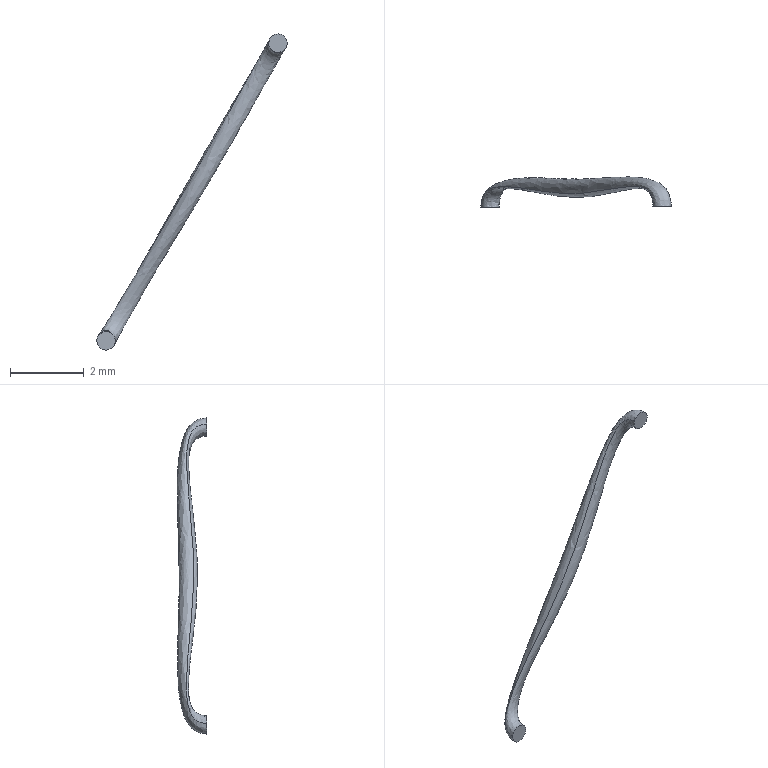Part | SolidWorks | features BaseBody 1 | 1 solid | 4 faces | box 5.15 x 0.8048 x 8.554 mm | volume 1.455 mm3 | plane 2 | spline 2
STEP:
#1=CARTESIAN_POINT('',(330.193,424.453,108.216));
#2=VERTEX_POINT('',#1);
#3=CARTESIAN_POINT('',(330.688,424.453,108.142));
#4=VERTEX_POINT('',#3);
#5=CARTESIAN_POINT('',(330.193,424.453,108.216));
#6=CARTESIAN_POINT('',(330.188,424.453,108.182));
#7=CARTESIAN_POINT('',(330.192,424.453,108.114));
#8=CARTESIAN_POINT('',(330.235,424.453,108.026));
#9=CARTESIAN_POINT('',(330.306,424.453,107.96));
#10=CARTESIAN_POINT('',(330.396,424.453,107.927));
#11=CARTESIAN_POINT('',(330.485,424.453,107.928));
#12=CARTESIAN_POINT('',(330.583,424.453,107.962));
#13=CARTESIAN_POINT('',(330.645,424.453,108.023));
#14=CARTESIAN_POINT('',(330.672,424.453,108.083));
#15=CARTESIAN_POINT('',(330.679,424.453,108.102));
#16=CARTESIAN_POINT('',(330.684,424.453,108.121));
#17=CARTESIAN_POINT('',(330.687,424.453,108.135));
#18=CARTESIAN_POINT('',(330.688,424.453,108.142));
#19=B_SPLINE_CURVE_WITH_KNOTS('',3,(#5,#6,#7,#8,#9,#10,#11,#12,#13,#14,#15,#16,#17,#18),.UNSPECIFIED.,.F.,.F.,(4,1,1,1,1,1,1,1,1,1,1,4),(0.,0.125,0.25,0.375,0.5,0.6,0.7,0.9,0.925,0.95,0.975,1.),.UNSPECIFIED.);
#20=EDGE_CURVE('',#2,#4,#19,.T.);
#21=ORIENTED_EDGE('',*,*,#20,.T.);
#22=CARTESIAN_POINT('',(330.688,424.453,108.142));
#23=CARTESIAN_POINT('',(330.689,424.453,108.148));
#24=CARTESIAN_POINT('',(330.69,424.453,108.162));
#25=CARTESIAN_POINT('',(330.691,424.453,108.182));
#26=CARTESIAN_POINT('',(330.69,424.453,108.202));
#27=CARTESIAN_POINT('',(330.681,424.453,108.267));
#28=CARTESIAN_POINT('',(330.64,424.453,108.344));
#29=CARTESIAN_POINT('',(330.557,424.453,108.405));
#30=CARTESIAN_POINT('',(330.472,424.453,108.432));
#31=CARTESIAN_POINT('',(330.376,424.453,108.427));
#32=CARTESIAN_POINT('',(330.289,424.453,108.384));
#33=CARTESIAN_POINT('',(330.222,424.453,108.313));
#34=CARTESIAN_POINT('',(330.198,424.453,108.249));
#35=CARTESIAN_POINT('',(330.193,424.453,108.216));
#36=B_SPLINE_CURVE_WITH_KNOTS('',3,(#22,#23,#24,#25,#26,#27,#28,#29,#30,#31,#32,#33,#34,#35),.UNSPECIFIED.,.F.,.F.,(4,1,1,1,1,1,1,1,1,1,1,4),(0.,0.025,0.05,0.075,0.1,0.3,0.4,0.5,0.625,0.75,0.875,1.),.UNSPECIFIED.);
#37=EDGE_CURVE('',#4,#2,#36,.T.);
#38=ORIENTED_EDGE('',*,*,#37,.T.);
#39=EDGE_LOOP('',(#21,#38));
#40=FACE_OUTER_BOUND('',#39,.T.);
#41=CARTESIAN_POINT('',(330.441,424.453,108.179));
#42=DIRECTION('',(-0.0009599,1.,0.));
#43=DIRECTION('',(0.,0.,1.));
#44=AXIS2_PLACEMENT_3D('',#41,#42,#43);
#45=PLANE('',#44);
#46=ADVANCED_FACE('',(#40),#45,.F.);
#47=CARTESIAN_POINT('',(334.856,424.457,116.318));
#48=VERTEX_POINT('',#47);
#49=CARTESIAN_POINT('',(335.326,424.458,116.148));
#50=VERTEX_POINT('',#49);
#51=CARTESIAN_POINT('',(334.856,424.457,116.318));
#52=CARTESIAN_POINT('',(334.844,424.457,116.286));
#53=CARTESIAN_POINT('',(334.835,424.457,116.219));
#54=CARTESIAN_POINT('',(334.859,424.457,116.124));
#55=CARTESIAN_POINT('',(334.916,424.457,116.045));
#56=CARTESIAN_POINT('',(334.998,424.457,115.995));
#57=CARTESIAN_POINT('',(335.085,424.457,115.979));
#58=CARTESIAN_POINT('',(335.188,424.458,115.993));
#59=CARTESIAN_POINT('',(335.26,424.458,116.041));
#60=CARTESIAN_POINT('',(335.299,424.458,116.094));
#61=CARTESIAN_POINT('',(335.309,424.458,116.111));
#62=CARTESIAN_POINT('',(335.318,424.458,116.129));
#63=CARTESIAN_POINT('',(335.324,424.458,116.142));
#64=CARTESIAN_POINT('',(335.326,424.458,116.148));
#65=B_SPLINE_CURVE_WITH_KNOTS('',3,(#51,#52,#53,#54,#55,#56,#57,#58,#59,#60,#61,#62,#63,#64),.UNSPECIFIED.,.F.,.F.,(4,1,1,1,1,1,1,1,1,1,1,4),(0.,0.125,0.25,0.375,0.5,0.6,0.7,0.9,0.925,0.95,0.975,1.),.UNSPECIFIED.);
#66=EDGE_CURVE('',#48,#50,#65,.T.);
#67=ORIENTED_EDGE('',*,*,#66,.T.);
#68=CARTESIAN_POINT('',(335.326,424.458,116.148));
#69=CARTESIAN_POINT('',(335.328,424.458,116.154));
#70=CARTESIAN_POINT('',(335.332,424.458,116.168));
#71=CARTESIAN_POINT('',(335.337,424.458,116.187));
#72=CARTESIAN_POINT('',(335.34,424.458,116.207));
#73=CARTESIAN_POINT('',(335.344,424.458,116.273));
#74=CARTESIAN_POINT('',(335.319,424.458,116.356));
#75=CARTESIAN_POINT('',(335.249,424.458,116.432));
#76=CARTESIAN_POINT('',(335.171,424.458,116.476));
#77=CARTESIAN_POINT('',(335.076,424.457,116.489));
#78=CARTESIAN_POINT('',(334.982,424.457,116.465));
#79=CARTESIAN_POINT('',(334.903,424.457,116.408));
#80=CARTESIAN_POINT('',(334.867,424.457,116.349));
#81=CARTESIAN_POINT('',(334.856,424.457,116.318));
#82=B_SPLINE_CURVE_WITH_KNOTS('',3,(#68,#69,#70,#71,#72,#73,#74,#75,#76,#77,#78,#79,#80,#81),.UNSPECIFIED.,.F.,.F.,(4,1,1,1,1,1,1,1,1,1,1,4),(0.,0.025,0.05,0.075,0.1,0.3,0.4,0.5,0.625,0.75,0.875,1.),.UNSPECIFIED.);
#83=EDGE_CURVE('',#50,#48,#82,.T.);
#84=ORIENTED_EDGE('',*,*,#83,.T.);
#85=EDGE_LOOP('',(#67,#84));
#86=FACE_OUTER_BOUND('',#85,.T.);
#87=CARTESIAN_POINT('',(335.091,424.457,116.233));
#88=DIRECTION('',(-0.0009599,1.,0.));
#89=DIRECTION('',(0.,0.,1.));
#90=AXIS2_PLACEMENT_3D('',#87,#88,#89);
#91=PLANE('',#90);
#92=ADVANCED_FACE('',(#86),#91,.F.);
#93=CARTESIAN_POINT('',(334.856,424.457,116.318));
#94=CARTESIAN_POINT('',(334.855,425.428,116.318));
#95=CARTESIAN_POINT('',(332.685,424.173,112.331));
#96=CARTESIAN_POINT('',(330.192,425.451,108.216));
#97=CARTESIAN_POINT('',(330.193,424.453,108.216));
#98=B_SPLINE_CURVE_WITH_KNOTS('',3,(#93,#94,#95,#96,#97),.UNSPECIFIED.,.F.,.F.,(4,1,4),(0.,0.5,1.),.UNSPECIFIED.);
#99=EDGE_CURVE('',#48,#2,#98,.T.);
#100=ORIENTED_EDGE('',*,*,#99,.T.);
#101=ORIENTED_EDGE('',*,*,#37,.F.);
#102=CARTESIAN_POINT('',(330.688,424.453,108.142));
#103=CARTESIAN_POINT('',(330.687,425.461,108.142));
#104=CARTESIAN_POINT('',(332.898,424.732,112.051));
#105=CARTESIAN_POINT('',(335.325,425.492,116.148));
#106=CARTESIAN_POINT('',(335.326,424.458,116.148));
#107=B_SPLINE_CURVE_WITH_KNOTS('',3,(#102,#103,#104,#105,#106),.UNSPECIFIED.,.F.,.F.,(4,1,4),(0.,0.5,1.),.UNSPECIFIED.);
#108=EDGE_CURVE('',#4,#50,#107,.T.);
#109=ORIENTED_EDGE('',*,*,#108,.T.);
#110=ORIENTED_EDGE('',*,*,#66,.F.);
#111=EDGE_LOOP('',(#100,#101,#109,#110));
#112=FACE_OUTER_BOUND('',#111,.T.);
#113=CARTESIAN_POINT('',(334.858,424.363,116.327));
#114=CARTESIAN_POINT('',(334.927,425.471,116.454));
#115=CARTESIAN_POINT('',(332.669,424.153,112.336));
#116=CARTESIAN_POINT('',(330.107,425.498,108.06));
#117=CARTESIAN_POINT('',(330.196,424.345,108.208));
#118=CARTESIAN_POINT('',(334.856,424.363,116.322));
#119=CARTESIAN_POINT('',(334.925,425.47,116.45));
#120=CARTESIAN_POINT('',(332.674,424.146,112.332));
#121=CARTESIAN_POINT('',(330.107,425.497,108.066));
#122=CARTESIAN_POINT('',(330.196,424.345,108.213));
#123=CARTESIAN_POINT('',(334.842,424.364,116.286));
#124=CARTESIAN_POINT('',(334.909,425.459,116.413));
#125=CARTESIAN_POINT('',(332.719,424.092,112.308));
#126=CARTESIAN_POINT('',(330.11,425.488,108.106));
#127=CARTESIAN_POINT('',(330.201,424.346,108.251));
#128=CARTESIAN_POINT('',(334.832,424.366,116.213));
#129=CARTESIAN_POINT('',(334.896,425.442,116.34));
#130=CARTESIAN_POINT('',(332.81,424.012,112.254));
#131=CARTESIAN_POINT('',(330.134,425.47,108.179));
#132=CARTESIAN_POINT('',(330.227,424.349,108.32));
#133=CARTESIAN_POINT('',(334.857,424.368,116.119));
#134=CARTESIAN_POINT('',(334.917,425.425,116.245));
#135=CARTESIAN_POINT('',(332.926,423.968,112.171));
#136=CARTESIAN_POINT('',(330.198,425.447,108.256));
#137=CARTESIAN_POINT('',(330.293,424.351,108.391));
#138=CARTESIAN_POINT('',(334.913,424.369,116.04));
#139=CARTESIAN_POINT('',(334.973,425.416,116.166));
#140=CARTESIAN_POINT('',(333.023,423.989,112.09));
#141=CARTESIAN_POINT('',(330.286,425.43,108.303));
#142=CARTESIAN_POINT('',(330.381,424.353,108.433));
#143=CARTESIAN_POINT('',(334.995,424.369,115.989));
#144=CARTESIAN_POINT('',(335.055,425.417,116.116));
#145=CARTESIAN_POINT('',(333.084,424.072,112.024));
#146=CARTESIAN_POINT('',(330.382,425.422,108.31));
#147=CARTESIAN_POINT('',(330.476,424.354,108.439));
#148=CARTESIAN_POINT('',(335.082,424.367,115.973));
#149=CARTESIAN_POINT('',(335.145,425.428,116.101));
#150=CARTESIAN_POINT('',(333.103,424.194,111.983));
#151=CARTESIAN_POINT('',(330.469,425.423,108.283));
#152=CARTESIAN_POINT('',(330.561,424.353,108.411));
#153=CARTESIAN_POINT('',(335.185,424.365,115.987));
#154=CARTESIAN_POINT('',(335.251,425.451,116.116));
#155=CARTESIAN_POINT('',(333.084,424.364,111.962));
#156=CARTESIAN_POINT('',(330.557,425.434,108.221));
#157=CARTESIAN_POINT('',(330.645,424.352,108.35));
#158=CARTESIAN_POINT('',(335.257,424.363,116.035));
#159=CARTESIAN_POINT('',(335.328,425.477,116.165));
#160=CARTESIAN_POINT('',(333.024,424.516,111.977));
#161=CARTESIAN_POINT('',(330.601,425.452,108.141));
#162=CARTESIAN_POINT('',(330.685,424.35,108.274));
#163=CARTESIAN_POINT('',(335.296,424.361,116.088));
#164=CARTESIAN_POINT('',(335.369,425.497,116.219));
#165=CARTESIAN_POINT('',(332.958,424.62,112.007));
#166=CARTESIAN_POINT('',(330.612,425.469,108.073));
#167=CARTESIAN_POINT('',(330.694,424.348,108.209));
#168=CARTESIAN_POINT('',(335.306,424.36,116.105));
#169=CARTESIAN_POINT('',(335.381,425.503,116.236));
#170=CARTESIAN_POINT('',(332.937,424.651,112.017));
#171=CARTESIAN_POINT('',(330.614,425.474,108.052));
#172=CARTESIAN_POINT('',(330.695,424.347,108.189));
#173=CARTESIAN_POINT('',(335.315,424.359,116.123));
#174=CARTESIAN_POINT('',(335.391,425.509,116.254));
#175=CARTESIAN_POINT('',(332.914,424.68,112.028));
#176=CARTESIAN_POINT('',(330.614,425.48,108.031));
#177=CARTESIAN_POINT('',(330.694,424.347,108.169));
#178=CARTESIAN_POINT('',(335.322,424.359,116.141));
#179=CARTESIAN_POINT('',(335.399,425.515,116.272));
#180=CARTESIAN_POINT('',(332.892,424.706,112.04));
#181=CARTESIAN_POINT('',(330.613,425.485,108.011));
#182=CARTESIAN_POINT('',(330.692,424.346,108.15));
#183=CARTESIAN_POINT('',(335.326,424.358,116.152));
#184=CARTESIAN_POINT('',(335.403,425.519,116.283));
#185=CARTESIAN_POINT('',(332.878,424.721,112.048));
#186=CARTESIAN_POINT('',(330.611,425.489,107.998));
#187=CARTESIAN_POINT('',(330.69,424.346,108.138));
#188=CARTESIAN_POINT('',(335.327,424.358,116.157));
#189=CARTESIAN_POINT('',(335.405,425.52,116.288));
#190=CARTESIAN_POINT('',(332.872,424.728,112.051));
#191=CARTESIAN_POINT('',(330.61,425.49,107.993));
#192=CARTESIAN_POINT('',(330.689,424.346,108.133));
#193=B_SPLINE_SURFACE_WITH_KNOTS('',3,3,((#113,#114,#115,#116,#117),(#118,#119,#120,#121,#122),(#123,#124,#125,#126,#127),(#128,#129,#130,#131,#132),(#133,#134,#135,#136,#137),(#138,#139,#140,#141,#142),(#143,#144,#145,#146,#147),(#148,#149,#150,#151,#152),(#153,#154,#155,#156,#157),(#158,#159,#160,#161,#162),(#163,#164,#165,#166,#167),(#168,#169,#170,#171,#172),(#173,#174,#175,#176,#177),(#178,#179,#180,#181,#182),(#183,#184,#185,#186,#187),(#188,#189,#190,#191,#192)),.UNSPECIFIED.,.F.,.F.,.F.,(4,1,1,1,1,1,1,1,1,1,1,1,1,4),(4,1,4),(0.4905,0.5,0.5625,0.625,0.6875,0.75,0.8,0.85,0.95,0.9625,0.975,0.9875,1.,1.01),(-0.01529,0.5,1.017),.UNSPECIFIED.);
#194=ADVANCED_FACE('',(#112),#193,.F.);
#195=ORIENTED_EDGE('',*,*,#83,.F.);
#196=ORIENTED_EDGE('',*,*,#108,.F.);
#197=ORIENTED_EDGE('',*,*,#20,.F.);
#198=ORIENTED_EDGE('',*,*,#99,.F.);
#199=EDGE_LOOP('',(#195,#196,#197,#198));
#200=FACE_OUTER_BOUND('',#199,.T.);
#201=CARTESIAN_POINT('',(335.317,424.359,116.128));
#202=CARTESIAN_POINT('',(335.393,425.511,116.259));
#203=CARTESIAN_POINT('',(332.909,424.687,112.031));
#204=CARTESIAN_POINT('',(330.613,425.481,108.026));
#205=CARTESIAN_POINT('',(330.694,424.347,108.164));
#206=CARTESIAN_POINT('',(335.319,424.359,116.132));
#207=CARTESIAN_POINT('',(335.395,425.512,116.263));
#208=CARTESIAN_POINT('',(332.903,424.694,112.034));
#209=CARTESIAN_POINT('',(330.613,425.483,108.02));
#210=CARTESIAN_POINT('',(330.693,424.346,108.159));
#211=CARTESIAN_POINT('',(335.323,424.359,116.144));
#212=CARTESIAN_POINT('',(335.4,425.516,116.275));
#213=CARTESIAN_POINT('',(332.889,424.71,112.042));
#214=CARTESIAN_POINT('',(330.612,425.486,108.008));
#215=CARTESIAN_POINT('',(330.692,424.346,108.147));
#216=CARTESIAN_POINT('',(335.329,424.358,116.162));
#217=CARTESIAN_POINT('',(335.407,425.522,116.293));
#218=CARTESIAN_POINT('',(332.866,424.734,112.055));
#219=CARTESIAN_POINT('',(330.609,425.492,107.988));
#220=CARTESIAN_POINT('',(330.688,424.345,108.128));
#221=CARTESIAN_POINT('',(335.334,424.358,116.181));
#222=CARTESIAN_POINT('',(335.412,425.527,116.313));
#223=CARTESIAN_POINT('',(332.842,424.758,112.069));
#224=CARTESIAN_POINT('',(330.604,425.497,107.967));
#225=CARTESIAN_POINT('',(330.683,424.345,108.109));
#226=CARTESIAN_POINT('',(335.336,424.357,116.201));
#227=CARTESIAN_POINT('',(335.416,425.533,116.333));
#228=CARTESIAN_POINT('',(332.817,424.779,112.084));
#229=CARTESIAN_POINT('',(330.598,425.503,107.947));
#230=CARTESIAN_POINT('',(330.676,424.344,108.09));
#231=CARTESIAN_POINT('',(335.34,424.355,116.267));
#232=CARTESIAN_POINT('',(335.423,425.55,116.399));
#233=CARTESIAN_POINT('',(332.736,424.841,112.134));
#234=CARTESIAN_POINT('',(330.572,425.521,107.884));
#235=CARTESIAN_POINT('',(330.648,424.342,108.031));
#236=CARTESIAN_POINT('',(335.315,424.354,116.35));
#237=CARTESIAN_POINT('',(335.4,425.565,116.482));
#238=CARTESIAN_POINT('',(332.634,424.873,112.208));
#239=CARTESIAN_POINT('',(330.512,425.542,107.818));
#240=CARTESIAN_POINT('',(330.587,424.34,107.97));
#241=CARTESIAN_POINT('',(335.245,424.354,116.426));
#242=CARTESIAN_POINT('',(335.33,425.569,116.559));
#243=CARTESIAN_POINT('',(332.54,424.831,112.291));
#244=CARTESIAN_POINT('',(330.414,425.557,107.78));
#245=CARTESIAN_POINT('',(330.489,424.338,107.936));
#246=CARTESIAN_POINT('',(335.168,424.354,116.47));
#247=CARTESIAN_POINT('',(335.252,425.565,116.602));
#248=CARTESIAN_POINT('',(332.487,424.749,112.351));
#249=CARTESIAN_POINT('',(330.324,425.562,107.777));
#250=CARTESIAN_POINT('',(330.4,424.338,107.935));
#251=CARTESIAN_POINT('',(335.073,424.355,116.483));
#252=CARTESIAN_POINT('',(335.155,425.55,116.614));
#253=CARTESIAN_POINT('',(332.472,424.616,112.392));
#254=CARTESIAN_POINT('',(330.232,425.557,107.81));
#255=CARTESIAN_POINT('',(330.31,424.339,107.968));
#256=CARTESIAN_POINT('',(334.979,424.358,116.459));
#257=CARTESIAN_POINT('',(335.057,425.524,116.589));
#258=CARTESIAN_POINT('',(332.503,424.453,112.402));
#259=CARTESIAN_POINT('',(330.157,425.541,107.878));
#260=CARTESIAN_POINT('',(330.239,424.34,108.034));
#261=CARTESIAN_POINT('',(334.9,424.361,116.402));
#262=CARTESIAN_POINT('',(334.973,425.495,116.531));
#263=CARTESIAN_POINT('',(332.574,424.284,112.382));
#264=CARTESIAN_POINT('',(330.111,425.519,107.969));
#265=CARTESIAN_POINT('',(330.197,424.343,108.121));
#266=CARTESIAN_POINT('',(334.861,424.363,116.339));
#267=CARTESIAN_POINT('',(334.931,425.474,116.467));
#268=CARTESIAN_POINT('',(332.653,424.169,112.345));
#269=CARTESIAN_POINT('',(330.104,425.502,108.047));
#270=CARTESIAN_POINT('',(330.193,424.345,108.195));
#271=CARTESIAN_POINT('',(334.849,424.364,116.303));
#272=CARTESIAN_POINT('',(334.917,425.464,116.43));
#273=CARTESIAN_POINT('',(332.698,424.118,112.319));
#274=CARTESIAN_POINT('',(330.109,425.492,108.087));
#275=CARTESIAN_POINT('',(330.2,424.346,108.233));
#276=CARTESIAN_POINT('',(334.848,424.364,116.298));
#277=CARTESIAN_POINT('',(334.916,425.463,116.425));
#278=CARTESIAN_POINT('',(332.704,424.112,112.316));
#279=CARTESIAN_POINT('',(330.11,425.491,108.092));
#280=CARTESIAN_POINT('',(330.201,424.346,108.238));
#281=B_SPLINE_SURFACE_WITH_KNOTS('',3,3,((#201,#202,#203,#204,#205),(#206,#207,#208,#209,#210),(#211,#212,#213,#214,#215),(#216,#217,#218,#219,#220),(#221,#222,#223,#224,#225),(#226,#227,#228,#229,#230),(#231,#232,#233,#234,#235),(#236,#237,#238,#239,#240),(#241,#242,#243,#244,#245),(#246,#247,#248,#249,#250),(#251,#252,#253,#254,#255),(#256,#257,#258,#259,#260),(#261,#262,#263,#264,#265),(#266,#267,#268,#269,#270),(#271,#272,#273,#274,#275),(#276,#277,#278,#279,#280)),.UNSPECIFIED.,.F.,.F.,.F.,(4,1,1,1,1,1,1,1,1,1,1,1,1,4),(4,1,4),(-0.009538,0.,0.0125,0.025,0.0375,0.05,0.15,0.2,0.25,0.3125,0.375,0.4375,0.5,0.5095),(-0.01529,0.5,1.017),.UNSPECIFIED.);
#282=ADVANCED_FACE('',(#200),#281,.F.);
#283=CLOSED_SHELL('',(#46,#92,#194,#282));
#284=MANIFOLD_SOLID_BREP('',#283);
#285=CARTESIAN_POINT('',(0.,0.,0.));
#286=DIRECTION('',(0.,0.,1.));
#287=DIRECTION('',(1.,0.,0.));
#288=AXIS2_PLACEMENT_3D('',#285,#286,#287);
#289=(LENGTH_UNIT()NAMED_UNIT(*)SI_UNIT(.MILLI.,.METRE.));
#290=UNCERTAINTY_MEASURE_WITH_UNIT(LENGTH_MEASURE(0.00001),#289,'','');
#291=(NAMED_UNIT(*)PLANE_ANGLE_UNIT()SI_UNIT($,.RADIAN.));
#292=(NAMED_UNIT(*)SI_UNIT($,.STERADIAN.)SOLID_ANGLE_UNIT());
#293=(GEOMETRIC_REPRESENTATION_CONTEXT(3)GLOBAL_UNCERTAINTY_ASSIGNED_CONTEXT((#290))GLOBAL_UNIT_ASSIGNED_CONTEXT((#289,#291,#292))REPRESENTATION_CONTEXT('',''));
#294=ADVANCED_BREP_SHAPE_REPRESENTATION('',(#284,#288),#293);